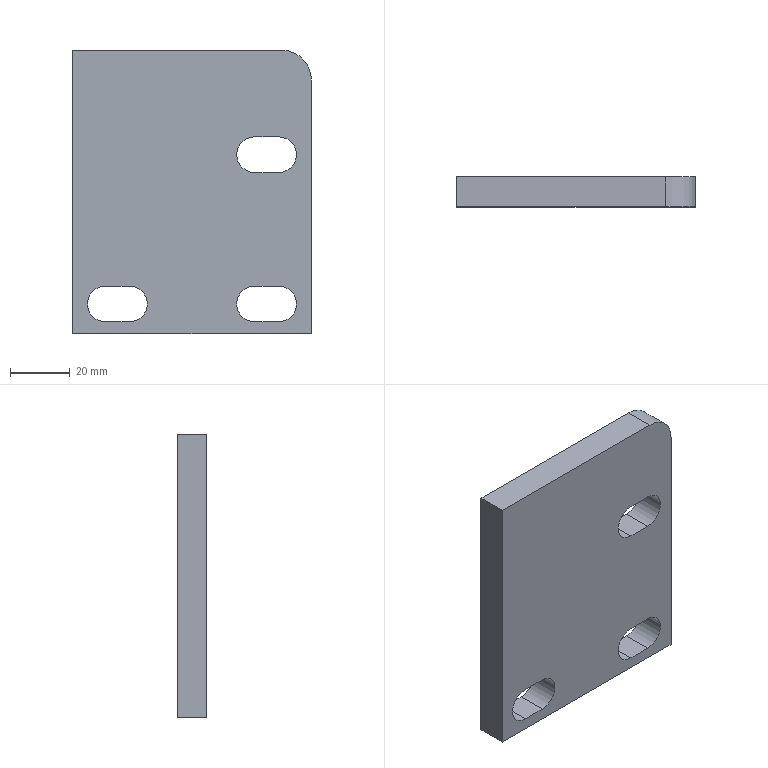Part | SolidWorks | features Extrusion 1 | 1 solid | 19 faces | box 80 x 10 x 95 mm | volume 69512 mm3 | plane 12 | cylinder 7 | commonest cylinder face diameters 12 x6 20 x1
STEP:
#1=CARTESIAN_POINT('',(40.,10.,37.5));
#2=VERTEX_POINT('',#1);
#3=CARTESIAN_POINT('',(40.,10.,-47.5));
#4=VERTEX_POINT('',#3);
#5=CARTESIAN_POINT('',(40.,10.,37.5));
#6=DIRECTION('',(0.,0.,-1.));
#7=VECTOR('',#6,1000.);
#8=LINE('',#5,#7);
#9=EDGE_CURVE('',#2,#4,#8,.T.);
#10=ORIENTED_EDGE('',*,*,#9,.T.);
#11=CARTESIAN_POINT('',(-40.,10.,-47.5));
#12=VERTEX_POINT('',#11);
#13=CARTESIAN_POINT('',(-40.,10.,-47.5));
#14=DIRECTION('',(-1.,0.,0.));
#15=VECTOR('',#14,1000.);
#16=LINE('',#13,#15);
#17=EDGE_CURVE('',#4,#12,#16,.T.);
#18=ORIENTED_EDGE('',*,*,#17,.T.);
#19=CARTESIAN_POINT('',(-40.,10.,47.5));
#20=VERTEX_POINT('',#19);
#21=CARTESIAN_POINT('',(-40.,10.,47.5));
#22=DIRECTION('',(0.,0.,1.));
#23=VECTOR('',#22,1000.);
#24=LINE('',#21,#23);
#25=EDGE_CURVE('',#12,#20,#24,.T.);
#26=ORIENTED_EDGE('',*,*,#25,.T.);
#27=CARTESIAN_POINT('',(30.,10.,47.5));
#28=VERTEX_POINT('',#27);
#29=CARTESIAN_POINT('',(-40.,10.,47.5));
#30=DIRECTION('',(1.,0.,0.));
#31=VECTOR('',#30,1000.);
#32=LINE('',#29,#31);
#33=EDGE_CURVE('',#20,#28,#32,.T.);
#34=ORIENTED_EDGE('',*,*,#33,.T.);
#35=CARTESIAN_POINT('',(30.,10.,37.5));
#36=DIRECTION('',(0.,1.,0.));
#37=DIRECTION('',(0.,0.,1.));
#38=AXIS2_PLACEMENT_3D('',#35,#36,#37);
#39=CIRCLE('',#38,10.);
#40=EDGE_CURVE('',#28,#2,#39,.T.);
#41=ORIENTED_EDGE('',*,*,#40,.T.);
#42=EDGE_LOOP('',(#10,#18,#26,#34,#41));
#43=FACE_OUTER_BOUND('',#42,.T.);
#44=CARTESIAN_POINT('',(-29.,10.,-31.5));
#45=VERTEX_POINT('',#44);
#46=CARTESIAN_POINT('',(-21.,10.,-31.5));
#47=VERTEX_POINT('',#46);
#48=CARTESIAN_POINT('',(-29.,10.,-31.5));
#49=DIRECTION('',(1.,0.,0.));
#50=VECTOR('',#49,1000.);
#51=LINE('',#48,#50);
#52=EDGE_CURVE('',#45,#47,#51,.T.);
#53=ORIENTED_EDGE('',*,*,#52,.F.);
#54=CARTESIAN_POINT('',(-29.,10.,-43.5));
#55=VERTEX_POINT('',#54);
#56=CARTESIAN_POINT('',(-29.,10.,-37.5));
#57=DIRECTION('',(0.,1.,0.));
#58=DIRECTION('',(0.,0.,1.));
#59=AXIS2_PLACEMENT_3D('',#56,#57,#58);
#60=CIRCLE('',#59,6.);
#61=EDGE_CURVE('',#55,#45,#60,.T.);
#62=ORIENTED_EDGE('',*,*,#61,.F.);
#63=CARTESIAN_POINT('',(-21.,10.,-43.5));
#64=VERTEX_POINT('',#63);
#65=CARTESIAN_POINT('',(-29.,10.,-43.5));
#66=DIRECTION('',(-1.,0.,0.));
#67=VECTOR('',#66,1000.);
#68=LINE('',#65,#67);
#69=EDGE_CURVE('',#64,#55,#68,.T.);
#70=ORIENTED_EDGE('',*,*,#69,.F.);
#71=CARTESIAN_POINT('',(-21.,10.,-37.5));
#72=DIRECTION('',(0.,1.,0.));
#73=DIRECTION('',(0.,0.,1.));
#74=AXIS2_PLACEMENT_3D('',#71,#72,#73);
#75=CIRCLE('',#74,6.);
#76=EDGE_CURVE('',#47,#64,#75,.T.);
#77=ORIENTED_EDGE('',*,*,#76,.F.);
#78=EDGE_LOOP('',(#53,#62,#70,#77));
#79=FACE_BOUND('',#78,.T.);
#80=CARTESIAN_POINT('',(21.,10.,-31.5));
#81=VERTEX_POINT('',#80);
#82=CARTESIAN_POINT('',(29.,10.,-31.5));
#83=VERTEX_POINT('',#82);
#84=CARTESIAN_POINT('',(21.,10.,-31.5));
#85=DIRECTION('',(1.,0.,0.));
#86=VECTOR('',#85,1000.);
#87=LINE('',#84,#86);
#88=EDGE_CURVE('',#81,#83,#87,.T.);
#89=ORIENTED_EDGE('',*,*,#88,.F.);
#90=CARTESIAN_POINT('',(21.,10.,-43.5));
#91=VERTEX_POINT('',#90);
#92=CARTESIAN_POINT('',(21.,10.,-37.5));
#93=DIRECTION('',(0.,1.,0.));
#94=DIRECTION('',(0.,0.,1.));
#95=AXIS2_PLACEMENT_3D('',#92,#93,#94);
#96=CIRCLE('',#95,6.);
#97=EDGE_CURVE('',#91,#81,#96,.T.);
#98=ORIENTED_EDGE('',*,*,#97,.F.);
#99=CARTESIAN_POINT('',(29.,10.,-43.5));
#100=VERTEX_POINT('',#99);
#101=CARTESIAN_POINT('',(21.,10.,-43.5));
#102=DIRECTION('',(-1.,0.,0.));
#103=VECTOR('',#102,1000.);
#104=LINE('',#101,#103);
#105=EDGE_CURVE('',#100,#91,#104,.T.);
#106=ORIENTED_EDGE('',*,*,#105,.F.);
#107=CARTESIAN_POINT('',(29.,10.,-37.5));
#108=DIRECTION('',(0.,1.,0.));
#109=DIRECTION('',(0.,0.,1.));
#110=AXIS2_PLACEMENT_3D('',#107,#108,#109);
#111=CIRCLE('',#110,6.);
#112=EDGE_CURVE('',#83,#100,#111,.T.);
#113=ORIENTED_EDGE('',*,*,#112,.F.);
#114=EDGE_LOOP('',(#89,#98,#106,#113));
#115=FACE_BOUND('',#114,.T.);
#116=CARTESIAN_POINT('',(21.,10.,18.5));
#117=VERTEX_POINT('',#116);
#118=CARTESIAN_POINT('',(29.,10.,18.5));
#119=VERTEX_POINT('',#118);
#120=CARTESIAN_POINT('',(21.,10.,18.5));
#121=DIRECTION('',(1.,0.,0.));
#122=VECTOR('',#121,1000.);
#123=LINE('',#120,#122);
#124=EDGE_CURVE('',#117,#119,#123,.T.);
#125=ORIENTED_EDGE('',*,*,#124,.F.);
#126=CARTESIAN_POINT('',(21.,10.,6.5));
#127=VERTEX_POINT('',#126);
#128=CARTESIAN_POINT('',(21.,10.,12.5));
#129=DIRECTION('',(0.,1.,0.));
#130=DIRECTION('',(0.,0.,1.));
#131=AXIS2_PLACEMENT_3D('',#128,#129,#130);
#132=CIRCLE('',#131,6.);
#133=EDGE_CURVE('',#127,#117,#132,.T.);
#134=ORIENTED_EDGE('',*,*,#133,.F.);
#135=CARTESIAN_POINT('',(29.,10.,6.5));
#136=VERTEX_POINT('',#135);
#137=CARTESIAN_POINT('',(21.,10.,6.5));
#138=DIRECTION('',(-1.,0.,0.));
#139=VECTOR('',#138,1000.);
#140=LINE('',#137,#139);
#141=EDGE_CURVE('',#136,#127,#140,.T.);
#142=ORIENTED_EDGE('',*,*,#141,.F.);
#143=CARTESIAN_POINT('',(29.,10.,12.5));
#144=DIRECTION('',(0.,1.,0.));
#145=DIRECTION('',(0.,0.,1.));
#146=AXIS2_PLACEMENT_3D('',#143,#144,#145);
#147=CIRCLE('',#146,6.);
#148=EDGE_CURVE('',#119,#136,#147,.T.);
#149=ORIENTED_EDGE('',*,*,#148,.F.);
#150=EDGE_LOOP('',(#125,#134,#142,#149));
#151=FACE_BOUND('',#150,.T.);
#152=CARTESIAN_POINT('',(30.,10.,37.5));
#153=DIRECTION('',(0.,1.,0.));
#154=DIRECTION('',(0.,0.,1.));
#155=AXIS2_PLACEMENT_3D('',#152,#153,#154);
#156=PLANE('',#155);
#157=ADVANCED_FACE('',(#43,#79,#115,#151),#156,.T.);
#158=CARTESIAN_POINT('',(21.,0.,-43.5));
#159=VERTEX_POINT('',#158);
#160=CARTESIAN_POINT('',(21.,0.,-31.5));
#161=VERTEX_POINT('',#160);
#162=CARTESIAN_POINT('',(21.,0.,-37.5));
#163=DIRECTION('',(0.,1.,0.));
#164=DIRECTION('',(0.,0.,1.));
#165=AXIS2_PLACEMENT_3D('',#162,#163,#164);
#166=CIRCLE('',#165,6.);
#167=EDGE_CURVE('',#159,#161,#166,.T.);
#168=ORIENTED_EDGE('',*,*,#167,.T.);
#169=CARTESIAN_POINT('',(29.,0.,-31.5));
#170=VERTEX_POINT('',#169);
#171=CARTESIAN_POINT('',(21.,0.,-31.5));
#172=DIRECTION('',(1.,0.,0.));
#173=VECTOR('',#172,1000.);
#174=LINE('',#171,#173);
#175=EDGE_CURVE('',#161,#170,#174,.T.);
#176=ORIENTED_EDGE('',*,*,#175,.T.);
#177=CARTESIAN_POINT('',(29.,0.,-43.5));
#178=VERTEX_POINT('',#177);
#179=CARTESIAN_POINT('',(29.,0.,-37.5));
#180=DIRECTION('',(0.,1.,0.));
#181=DIRECTION('',(0.,0.,1.));
#182=AXIS2_PLACEMENT_3D('',#179,#180,#181);
#183=CIRCLE('',#182,6.);
#184=EDGE_CURVE('',#170,#178,#183,.T.);
#185=ORIENTED_EDGE('',*,*,#184,.T.);
#186=CARTESIAN_POINT('',(21.,0.,-43.5));
#187=DIRECTION('',(-1.,0.,0.));
#188=VECTOR('',#187,1000.);
#189=LINE('',#186,#188);
#190=EDGE_CURVE('',#178,#159,#189,.T.);
#191=ORIENTED_EDGE('',*,*,#190,.T.);
#192=EDGE_LOOP('',(#168,#176,#185,#191));
#193=FACE_BOUND('',#192,.T.);
#194=CARTESIAN_POINT('',(40.,0.,37.5));
#195=VERTEX_POINT('',#194);
#196=CARTESIAN_POINT('',(40.,0.,-47.5));
#197=VERTEX_POINT('',#196);
#198=CARTESIAN_POINT('',(40.,0.,37.5));
#199=DIRECTION('',(0.,0.,-1.));
#200=VECTOR('',#199,1000.);
#201=LINE('',#198,#200);
#202=EDGE_CURVE('',#195,#197,#201,.T.);
#203=ORIENTED_EDGE('',*,*,#202,.F.);
#204=CARTESIAN_POINT('',(30.,0.,47.5));
#205=VERTEX_POINT('',#204);
#206=CARTESIAN_POINT('',(30.,0.,37.5));
#207=DIRECTION('',(0.,1.,0.));
#208=DIRECTION('',(0.,0.,1.));
#209=AXIS2_PLACEMENT_3D('',#206,#207,#208);
#210=CIRCLE('',#209,10.);
#211=EDGE_CURVE('',#205,#195,#210,.T.);
#212=ORIENTED_EDGE('',*,*,#211,.F.);
#213=CARTESIAN_POINT('',(-40.,0.,47.5));
#214=VERTEX_POINT('',#213);
#215=CARTESIAN_POINT('',(-40.,0.,47.5));
#216=DIRECTION('',(1.,0.,0.));
#217=VECTOR('',#216,1000.);
#218=LINE('',#215,#217);
#219=EDGE_CURVE('',#214,#205,#218,.T.);
#220=ORIENTED_EDGE('',*,*,#219,.F.);
#221=CARTESIAN_POINT('',(-40.,0.,-47.5));
#222=VERTEX_POINT('',#221);
#223=CARTESIAN_POINT('',(-40.,0.,47.5));
#224=DIRECTION('',(0.,0.,1.));
#225=VECTOR('',#224,1000.);
#226=LINE('',#223,#225);
#227=EDGE_CURVE('',#222,#214,#226,.T.);
#228=ORIENTED_EDGE('',*,*,#227,.F.);
#229=CARTESIAN_POINT('',(-40.,0.,-47.5));
#230=DIRECTION('',(-1.,0.,0.));
#231=VECTOR('',#230,1000.);
#232=LINE('',#229,#231);
#233=EDGE_CURVE('',#197,#222,#232,.T.);
#234=ORIENTED_EDGE('',*,*,#233,.F.);
#235=EDGE_LOOP('',(#203,#212,#220,#228,#234));
#236=FACE_OUTER_BOUND('',#235,.T.);
#237=CARTESIAN_POINT('',(-29.,0.,-43.5));
#238=VERTEX_POINT('',#237);
#239=CARTESIAN_POINT('',(-29.,0.,-31.5));
#240=VERTEX_POINT('',#239);
#241=CARTESIAN_POINT('',(-29.,0.,-37.5));
#242=DIRECTION('',(0.,1.,0.));
#243=DIRECTION('',(0.,0.,1.));
#244=AXIS2_PLACEMENT_3D('',#241,#242,#243);
#245=CIRCLE('',#244,6.);
#246=EDGE_CURVE('',#238,#240,#245,.T.);
#247=ORIENTED_EDGE('',*,*,#246,.T.);
#248=CARTESIAN_POINT('',(-21.,0.,-31.5));
#249=VERTEX_POINT('',#248);
#250=CARTESIAN_POINT('',(-29.,0.,-31.5));
#251=DIRECTION('',(1.,0.,0.));
#252=VECTOR('',#251,1000.);
#253=LINE('',#250,#252);
#254=EDGE_CURVE('',#240,#249,#253,.T.);
#255=ORIENTED_EDGE('',*,*,#254,.T.);
#256=CARTESIAN_POINT('',(-21.,0.,-43.5));
#257=VERTEX_POINT('',#256);
#258=CARTESIAN_POINT('',(-21.,0.,-37.5));
#259=DIRECTION('',(0.,1.,0.));
#260=DIRECTION('',(0.,0.,1.));
#261=AXIS2_PLACEMENT_3D('',#258,#259,#260);
#262=CIRCLE('',#261,6.);
#263=EDGE_CURVE('',#249,#257,#262,.T.);
#264=ORIENTED_EDGE('',*,*,#263,.T.);
#265=CARTESIAN_POINT('',(-29.,0.,-43.5));
#266=DIRECTION('',(-1.,0.,0.));
#267=VECTOR('',#266,1000.);
#268=LINE('',#265,#267);
#269=EDGE_CURVE('',#257,#238,#268,.T.);
#270=ORIENTED_EDGE('',*,*,#269,.T.);
#271=EDGE_LOOP('',(#247,#255,#264,#270));
#272=FACE_BOUND('',#271,.T.);
#273=CARTESIAN_POINT('',(21.,0.,6.5));
#274=VERTEX_POINT('',#273);
#275=CARTESIAN_POINT('',(21.,0.,18.5));
#276=VERTEX_POINT('',#275);
#277=CARTESIAN_POINT('',(21.,0.,12.5));
#278=DIRECTION('',(0.,1.,0.));
#279=DIRECTION('',(0.,0.,1.));
#280=AXIS2_PLACEMENT_3D('',#277,#278,#279);
#281=CIRCLE('',#280,6.);
#282=EDGE_CURVE('',#274,#276,#281,.T.);
#283=ORIENTED_EDGE('',*,*,#282,.T.);
#284=CARTESIAN_POINT('',(29.,0.,18.5));
#285=VERTEX_POINT('',#284);
#286=CARTESIAN_POINT('',(21.,0.,18.5));
#287=DIRECTION('',(1.,0.,0.));
#288=VECTOR('',#287,1000.);
#289=LINE('',#286,#288);
#290=EDGE_CURVE('',#276,#285,#289,.T.);
#291=ORIENTED_EDGE('',*,*,#290,.T.);
#292=CARTESIAN_POINT('',(29.,0.,6.5));
#293=VERTEX_POINT('',#292);
#294=CARTESIAN_POINT('',(29.,0.,12.5));
#295=DIRECTION('',(0.,1.,0.));
#296=DIRECTION('',(0.,0.,1.));
#297=AXIS2_PLACEMENT_3D('',#294,#295,#296);
#298=CIRCLE('',#297,6.);
#299=EDGE_CURVE('',#285,#293,#298,.T.);
#300=ORIENTED_EDGE('',*,*,#299,.T.);
#301=CARTESIAN_POINT('',(21.,0.,6.5));
#302=DIRECTION('',(-1.,0.,0.));
#303=VECTOR('',#302,1000.);
#304=LINE('',#301,#303);
#305=EDGE_CURVE('',#293,#274,#304,.T.);
#306=ORIENTED_EDGE('',*,*,#305,.T.);
#307=EDGE_LOOP('',(#283,#291,#300,#306));
#308=FACE_BOUND('',#307,.T.);
#309=CARTESIAN_POINT('',(30.,0.,37.5));
#310=DIRECTION('',(0.,1.,0.));
#311=DIRECTION('',(0.,0.,1.));
#312=AXIS2_PLACEMENT_3D('',#309,#310,#311);
#313=PLANE('',#312);
#314=ADVANCED_FACE('',(#193,#236,#272,#308),#313,.F.);
#315=ORIENTED_EDGE('',*,*,#202,.T.);
#316=CARTESIAN_POINT('',(40.,10.,-47.5));
#317=DIRECTION('',(0.,-1.,0.));
#318=VECTOR('',#317,1000.);
#319=LINE('',#316,#318);
#320=EDGE_CURVE('',#4,#197,#319,.T.);
#321=ORIENTED_EDGE('',*,*,#320,.F.);
#322=ORIENTED_EDGE('',*,*,#9,.F.);
#323=CARTESIAN_POINT('',(40.,10.,37.5));
#324=DIRECTION('',(0.,-1.,0.));
#325=VECTOR('',#324,1000.);
#326=LINE('',#323,#325);
#327=EDGE_CURVE('',#2,#195,#326,.T.);
#328=ORIENTED_EDGE('',*,*,#327,.T.);
#329=EDGE_LOOP('',(#315,#321,#322,#328));
#330=FACE_OUTER_BOUND('',#329,.T.);
#331=CARTESIAN_POINT('',(40.,10.,37.5));
#332=DIRECTION('',(-1.,0.,0.));
#333=DIRECTION('',(0.,0.,1.));
#334=AXIS2_PLACEMENT_3D('',#331,#332,#333);
#335=PLANE('',#334);
#336=ADVANCED_FACE('',(#330),#335,.F.);
#337=ORIENTED_EDGE('',*,*,#233,.T.);
#338=CARTESIAN_POINT('',(-40.,10.,-47.5));
#339=DIRECTION('',(0.,-1.,0.));
#340=VECTOR('',#339,1000.);
#341=LINE('',#338,#340);
#342=EDGE_CURVE('',#12,#222,#341,.T.);
#343=ORIENTED_EDGE('',*,*,#342,.F.);
#344=ORIENTED_EDGE('',*,*,#17,.F.);
#345=ORIENTED_EDGE('',*,*,#320,.T.);
#346=EDGE_LOOP('',(#337,#343,#344,#345));
#347=FACE_OUTER_BOUND('',#346,.T.);
#348=CARTESIAN_POINT('',(-40.,10.,-47.5));
#349=DIRECTION('',(0.,0.,1.));
#350=DIRECTION('',(1.,0.,0.));
#351=AXIS2_PLACEMENT_3D('',#348,#349,#350);
#352=PLANE('',#351);
#353=ADVANCED_FACE('',(#347),#352,.F.);
#354=ORIENTED_EDGE('',*,*,#227,.T.);
#355=CARTESIAN_POINT('',(-40.,10.,47.5));
#356=DIRECTION('',(0.,-1.,0.));
#357=VECTOR('',#356,1000.);
#358=LINE('',#355,#357);
#359=EDGE_CURVE('',#20,#214,#358,.T.);
#360=ORIENTED_EDGE('',*,*,#359,.F.);
#361=ORIENTED_EDGE('',*,*,#25,.F.);
#362=ORIENTED_EDGE('',*,*,#342,.T.);
#363=EDGE_LOOP('',(#354,#360,#361,#362));
#364=FACE_OUTER_BOUND('',#363,.T.);
#365=CARTESIAN_POINT('',(-40.,10.,47.5));
#366=DIRECTION('',(1.,0.,0.));
#367=DIRECTION('',(0.,0.,-1.));
#368=AXIS2_PLACEMENT_3D('',#365,#366,#367);
#369=PLANE('',#368);
#370=ADVANCED_FACE('',(#364),#369,.F.);
#371=ORIENTED_EDGE('',*,*,#219,.T.);
#372=CARTESIAN_POINT('',(30.,10.,47.5));
#373=DIRECTION('',(0.,-1.,0.));
#374=VECTOR('',#373,1000.);
#375=LINE('',#372,#374);
#376=EDGE_CURVE('',#28,#205,#375,.T.);
#377=ORIENTED_EDGE('',*,*,#376,.F.);
#378=ORIENTED_EDGE('',*,*,#33,.F.);
#379=ORIENTED_EDGE('',*,*,#359,.T.);
#380=EDGE_LOOP('',(#371,#377,#378,#379));
#381=FACE_OUTER_BOUND('',#380,.T.);
#382=CARTESIAN_POINT('',(-40.,10.,47.5));
#383=DIRECTION('',(0.,0.,-1.));
#384=DIRECTION('',(-1.,0.,0.));
#385=AXIS2_PLACEMENT_3D('',#382,#383,#384);
#386=PLANE('',#385);
#387=ADVANCED_FACE('',(#381),#386,.F.);
#388=ORIENTED_EDGE('',*,*,#211,.T.);
#389=ORIENTED_EDGE('',*,*,#327,.F.);
#390=ORIENTED_EDGE('',*,*,#40,.F.);
#391=ORIENTED_EDGE('',*,*,#376,.T.);
#392=EDGE_LOOP('',(#388,#389,#390,#391));
#393=FACE_OUTER_BOUND('',#392,.T.);
#394=CARTESIAN_POINT('',(30.,10.,37.5));
#395=DIRECTION('',(0.,-1.,0.));
#396=DIRECTION('',(0.,0.,-1.));
#397=AXIS2_PLACEMENT_3D('',#394,#395,#396);
#398=CYLINDRICAL_SURFACE('',#397,10.);
#399=ADVANCED_FACE('',(#393),#398,.T.);
#400=ORIENTED_EDGE('',*,*,#246,.F.);
#401=CARTESIAN_POINT('',(-29.,10.,-43.5));
#402=DIRECTION('',(0.,-1.,0.));
#403=VECTOR('',#402,1000.);
#404=LINE('',#401,#403);
#405=EDGE_CURVE('',#55,#238,#404,.T.);
#406=ORIENTED_EDGE('',*,*,#405,.F.);
#407=ORIENTED_EDGE('',*,*,#61,.T.);
#408=CARTESIAN_POINT('',(-29.,10.,-31.5));
#409=DIRECTION('',(0.,-1.,0.));
#410=VECTOR('',#409,1000.);
#411=LINE('',#408,#410);
#412=EDGE_CURVE('',#45,#240,#411,.T.);
#413=ORIENTED_EDGE('',*,*,#412,.T.);
#414=EDGE_LOOP('',(#400,#406,#407,#413));
#415=FACE_OUTER_BOUND('',#414,.T.);
#416=CARTESIAN_POINT('',(-29.,10.,-37.5));
#417=DIRECTION('',(0.,-1.,0.));
#418=DIRECTION('',(0.,0.,-1.));
#419=AXIS2_PLACEMENT_3D('',#416,#417,#418);
#420=CYLINDRICAL_SURFACE('',#419,6.);
#421=ADVANCED_FACE('',(#415),#420,.F.);
#422=ORIENTED_EDGE('',*,*,#254,.F.);
#423=ORIENTED_EDGE('',*,*,#412,.F.);
#424=ORIENTED_EDGE('',*,*,#52,.T.);
#425=CARTESIAN_POINT('',(-21.,10.,-31.5));
#426=DIRECTION('',(0.,-1.,0.));
#427=VECTOR('',#426,1000.);
#428=LINE('',#425,#427);
#429=EDGE_CURVE('',#47,#249,#428,.T.);
#430=ORIENTED_EDGE('',*,*,#429,.T.);
#431=EDGE_LOOP('',(#422,#423,#424,#430));
#432=FACE_OUTER_BOUND('',#431,.T.);
#433=CARTESIAN_POINT('',(-29.,10.,-31.5));
#434=DIRECTION('',(0.,0.,-1.));
#435=DIRECTION('',(-1.,0.,0.));
#436=AXIS2_PLACEMENT_3D('',#433,#434,#435);
#437=PLANE('',#436);
#438=ADVANCED_FACE('',(#432),#437,.T.);
#439=ORIENTED_EDGE('',*,*,#263,.F.);
#440=ORIENTED_EDGE('',*,*,#429,.F.);
#441=ORIENTED_EDGE('',*,*,#76,.T.);
#442=CARTESIAN_POINT('',(-21.,10.,-43.5));
#443=DIRECTION('',(0.,-1.,0.));
#444=VECTOR('',#443,1000.);
#445=LINE('',#442,#444);
#446=EDGE_CURVE('',#64,#257,#445,.T.);
#447=ORIENTED_EDGE('',*,*,#446,.T.);
#448=EDGE_LOOP('',(#439,#440,#441,#447));
#449=FACE_OUTER_BOUND('',#448,.T.);
#450=CARTESIAN_POINT('',(-21.,10.,-37.5));
#451=DIRECTION('',(0.,-1.,0.));
#452=DIRECTION('',(0.,0.,-1.));
#453=AXIS2_PLACEMENT_3D('',#450,#451,#452);
#454=CYLINDRICAL_SURFACE('',#453,6.);
#455=ADVANCED_FACE('',(#449),#454,.F.);
#456=ORIENTED_EDGE('',*,*,#269,.F.);
#457=ORIENTED_EDGE('',*,*,#446,.F.);
#458=ORIENTED_EDGE('',*,*,#69,.T.);
#459=ORIENTED_EDGE('',*,*,#405,.T.);
#460=EDGE_LOOP('',(#456,#457,#458,#459));
#461=FACE_OUTER_BOUND('',#460,.T.);
#462=CARTESIAN_POINT('',(-29.,10.,-43.5));
#463=DIRECTION('',(0.,0.,1.));
#464=DIRECTION('',(1.,0.,0.));
#465=AXIS2_PLACEMENT_3D('',#462,#463,#464);
#466=PLANE('',#465);
#467=ADVANCED_FACE('',(#461),#466,.T.);
#468=ORIENTED_EDGE('',*,*,#167,.F.);
#469=CARTESIAN_POINT('',(21.,10.,-43.5));
#470=DIRECTION('',(0.,-1.,0.));
#471=VECTOR('',#470,1000.);
#472=LINE('',#469,#471);
#473=EDGE_CURVE('',#91,#159,#472,.T.);
#474=ORIENTED_EDGE('',*,*,#473,.F.);
#475=ORIENTED_EDGE('',*,*,#97,.T.);
#476=CARTESIAN_POINT('',(21.,10.,-31.5));
#477=DIRECTION('',(0.,-1.,0.));
#478=VECTOR('',#477,1000.);
#479=LINE('',#476,#478);
#480=EDGE_CURVE('',#81,#161,#479,.T.);
#481=ORIENTED_EDGE('',*,*,#480,.T.);
#482=EDGE_LOOP('',(#468,#474,#475,#481));
#483=FACE_OUTER_BOUND('',#482,.T.);
#484=CARTESIAN_POINT('',(21.,10.,-37.5));
#485=DIRECTION('',(0.,-1.,0.));
#486=DIRECTION('',(0.,0.,-1.));
#487=AXIS2_PLACEMENT_3D('',#484,#485,#486);
#488=CYLINDRICAL_SURFACE('',#487,6.);
#489=ADVANCED_FACE('',(#483),#488,.F.);
#490=ORIENTED_EDGE('',*,*,#175,.F.);
#491=ORIENTED_EDGE('',*,*,#480,.F.);
#492=ORIENTED_EDGE('',*,*,#88,.T.);
#493=CARTESIAN_POINT('',(29.,10.,-31.5));
#494=DIRECTION('',(0.,-1.,0.));
#495=VECTOR('',#494,1000.);
#496=LINE('',#493,#495);
#497=EDGE_CURVE('',#83,#170,#496,.T.);
#498=ORIENTED_EDGE('',*,*,#497,.T.);
#499=EDGE_LOOP('',(#490,#491,#492,#498));
#500=FACE_OUTER_BOUND('',#499,.T.);
#501=CARTESIAN_POINT('',(21.,10.,-31.5));
#502=DIRECTION('',(0.,0.,-1.));
#503=DIRECTION('',(-1.,0.,0.));
#504=AXIS2_PLACEMENT_3D('',#501,#502,#503);
#505=PLANE('',#504);
#506=ADVANCED_FACE('',(#500),#505,.T.);
#507=ORIENTED_EDGE('',*,*,#184,.F.);
#508=ORIENTED_EDGE('',*,*,#497,.F.);
#509=ORIENTED_EDGE('',*,*,#112,.T.);
#510=CARTESIAN_POINT('',(29.,10.,-43.5));
#511=DIRECTION('',(0.,-1.,0.));
#512=VECTOR('',#511,1000.);
#513=LINE('',#510,#512);
#514=EDGE_CURVE('',#100,#178,#513,.T.);
#515=ORIENTED_EDGE('',*,*,#514,.T.);
#516=EDGE_LOOP('',(#507,#508,#509,#515));
#517=FACE_OUTER_BOUND('',#516,.T.);
#518=CARTESIAN_POINT('',(29.,10.,-37.5));
#519=DIRECTION('',(0.,-1.,0.));
#520=DIRECTION('',(0.,0.,-1.));
#521=AXIS2_PLACEMENT_3D('',#518,#519,#520);
#522=CYLINDRICAL_SURFACE('',#521,6.);
#523=ADVANCED_FACE('',(#517),#522,.F.);
#524=ORIENTED_EDGE('',*,*,#190,.F.);
#525=ORIENTED_EDGE('',*,*,#514,.F.);
#526=ORIENTED_EDGE('',*,*,#105,.T.);
#527=ORIENTED_EDGE('',*,*,#473,.T.);
#528=EDGE_LOOP('',(#524,#525,#526,#527));
#529=FACE_OUTER_BOUND('',#528,.T.);
#530=CARTESIAN_POINT('',(21.,10.,-43.5));
#531=DIRECTION('',(0.,0.,1.));
#532=DIRECTION('',(1.,0.,0.));
#533=AXIS2_PLACEMENT_3D('',#530,#531,#532);
#534=PLANE('',#533);
#535=ADVANCED_FACE('',(#529),#534,.T.);
#536=ORIENTED_EDGE('',*,*,#282,.F.);
#537=CARTESIAN_POINT('',(21.,10.,6.5));
#538=DIRECTION('',(0.,-1.,0.));
#539=VECTOR('',#538,1000.);
#540=LINE('',#537,#539);
#541=EDGE_CURVE('',#127,#274,#540,.T.);
#542=ORIENTED_EDGE('',*,*,#541,.F.);
#543=ORIENTED_EDGE('',*,*,#133,.T.);
#544=CARTESIAN_POINT('',(21.,10.,18.5));
#545=DIRECTION('',(0.,-1.,0.));
#546=VECTOR('',#545,1000.);
#547=LINE('',#544,#546);
#548=EDGE_CURVE('',#117,#276,#547,.T.);
#549=ORIENTED_EDGE('',*,*,#548,.T.);
#550=EDGE_LOOP('',(#536,#542,#543,#549));
#551=FACE_OUTER_BOUND('',#550,.T.);
#552=CARTESIAN_POINT('',(21.,10.,12.5));
#553=DIRECTION('',(0.,-1.,0.));
#554=DIRECTION('',(0.,0.,-1.));
#555=AXIS2_PLACEMENT_3D('',#552,#553,#554);
#556=CYLINDRICAL_SURFACE('',#555,6.);
#557=ADVANCED_FACE('',(#551),#556,.F.);
#558=ORIENTED_EDGE('',*,*,#290,.F.);
#559=ORIENTED_EDGE('',*,*,#548,.F.);
#560=ORIENTED_EDGE('',*,*,#124,.T.);
#561=CARTESIAN_POINT('',(29.,10.,18.5));
#562=DIRECTION('',(0.,-1.,0.));
#563=VECTOR('',#562,1000.);
#564=LINE('',#561,#563);
#565=EDGE_CURVE('',#119,#285,#564,.T.);
#566=ORIENTED_EDGE('',*,*,#565,.T.);
#567=EDGE_LOOP('',(#558,#559,#560,#566));
#568=FACE_OUTER_BOUND('',#567,.T.);
#569=CARTESIAN_POINT('',(21.,10.,18.5));
#570=DIRECTION('',(0.,0.,-1.));
#571=DIRECTION('',(-1.,0.,0.));
#572=AXIS2_PLACEMENT_3D('',#569,#570,#571);
#573=PLANE('',#572);
#574=ADVANCED_FACE('',(#568),#573,.T.);
#575=ORIENTED_EDGE('',*,*,#299,.F.);
#576=ORIENTED_EDGE('',*,*,#565,.F.);
#577=ORIENTED_EDGE('',*,*,#148,.T.);
#578=CARTESIAN_POINT('',(29.,10.,6.5));
#579=DIRECTION('',(0.,-1.,0.));
#580=VECTOR('',#579,1000.);
#581=LINE('',#578,#580);
#582=EDGE_CURVE('',#136,#293,#581,.T.);
#583=ORIENTED_EDGE('',*,*,#582,.T.);
#584=EDGE_LOOP('',(#575,#576,#577,#583));
#585=FACE_OUTER_BOUND('',#584,.T.);
#586=CARTESIAN_POINT('',(29.,10.,12.5));
#587=DIRECTION('',(0.,-1.,0.));
#588=DIRECTION('',(0.,0.,-1.));
#589=AXIS2_PLACEMENT_3D('',#586,#587,#588);
#590=CYLINDRICAL_SURFACE('',#589,6.);
#591=ADVANCED_FACE('',(#585),#590,.F.);
#592=ORIENTED_EDGE('',*,*,#305,.F.);
#593=ORIENTED_EDGE('',*,*,#582,.F.);
#594=ORIENTED_EDGE('',*,*,#141,.T.);
#595=ORIENTED_EDGE('',*,*,#541,.T.);
#596=EDGE_LOOP('',(#592,#593,#594,#595));
#597=FACE_OUTER_BOUND('',#596,.T.);
#598=CARTESIAN_POINT('',(21.,10.,6.5));
#599=DIRECTION('',(0.,0.,1.));
#600=DIRECTION('',(1.,0.,0.));
#601=AXIS2_PLACEMENT_3D('',#598,#599,#600);
#602=PLANE('',#601);
#603=ADVANCED_FACE('',(#597),#602,.T.);
#604=CLOSED_SHELL('',(#157,#314,#336,#353,#370,#387,#399,#421,#438,#455,#467,#489,#506,#523,#535,#557,#574,#591,#603));
#605=MANIFOLD_SOLID_BREP('',#604);
#606=CARTESIAN_POINT('',(0.,0.,0.));
#607=DIRECTION('',(0.,0.,1.));
#608=DIRECTION('',(1.,0.,0.));
#609=AXIS2_PLACEMENT_3D('',#606,#607,#608);
#610=(LENGTH_UNIT()NAMED_UNIT(*)SI_UNIT(.MILLI.,.METRE.));
#611=UNCERTAINTY_MEASURE_WITH_UNIT(LENGTH_MEASURE(0.00001),#610,'','');
#612=(NAMED_UNIT(*)PLANE_ANGLE_UNIT()SI_UNIT($,.RADIAN.));
#613=(NAMED_UNIT(*)SI_UNIT($,.STERADIAN.)SOLID_ANGLE_UNIT());
#614=(GEOMETRIC_REPRESENTATION_CONTEXT(3)GLOBAL_UNCERTAINTY_ASSIGNED_CONTEXT((#611))GLOBAL_UNIT_ASSIGNED_CONTEXT((#610,#612,#613))REPRESENTATION_CONTEXT('',''));
#615=ADVANCED_BREP_SHAPE_REPRESENTATION('',(#605,#609),#614);